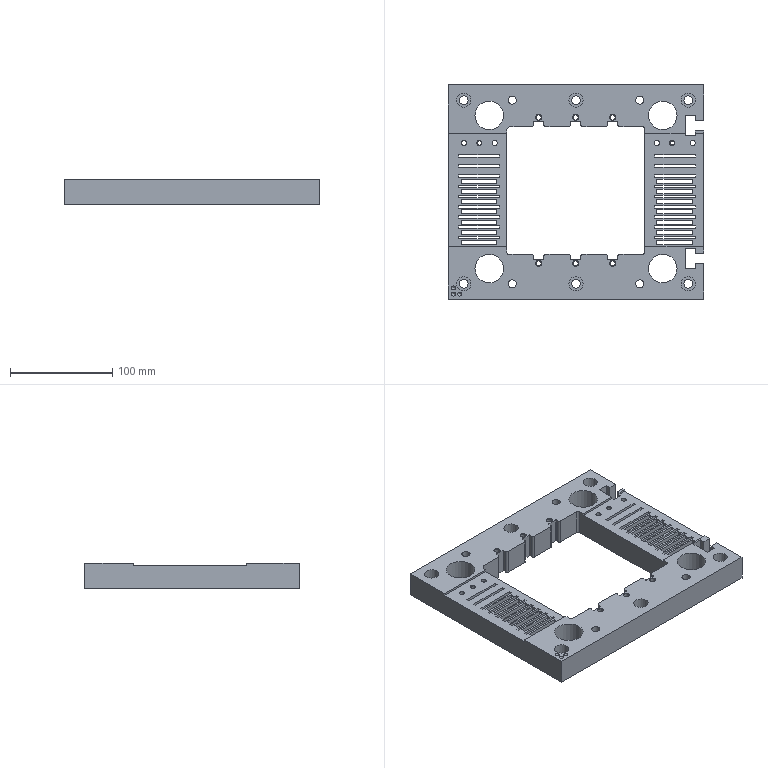Part | STEP file | 200 mesh_id2026 | 1 solid | 273 faces | box 250 x 210 x 25 mm | volume 669439 mm3 | plane 194 | cylinder 59 | cone 20 | commonest cylinder face diameters 1.03 x12 3.97 x12 5 x6 8.6 x6 14 x6 5.02 x4